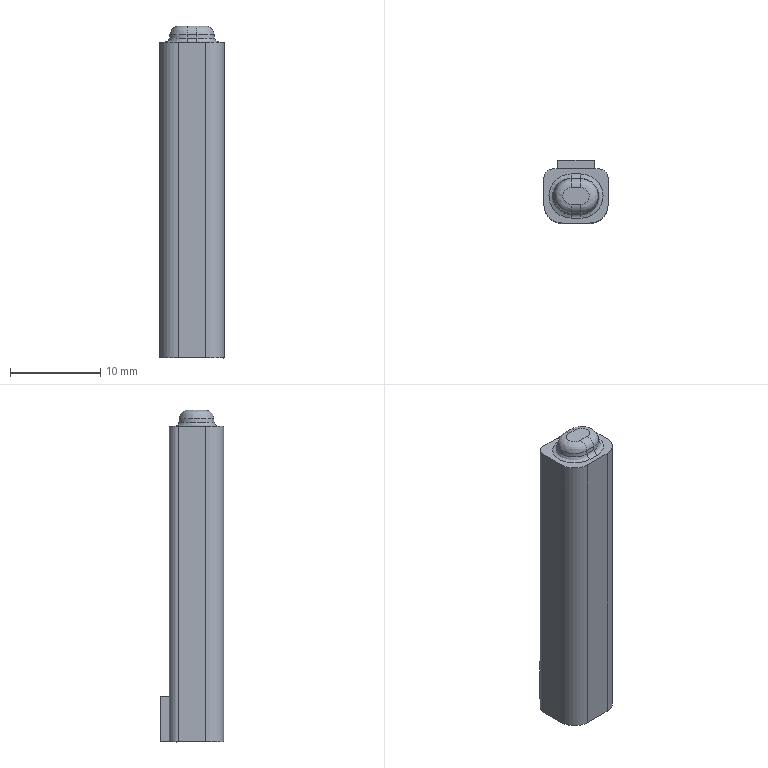Part | NX | features DIE-100 2 | 1 solid | 27 faces | box 7.1 x 7 x 36.8 mm | volume 1462 mm3 | plane 13 | cylinder 8 | spline 6 | commonest cylinder face diameters 2 x4 1 x2 4 x2
STEP:
#1=CARTESIAN_POINT('',(4190.723,-837.209,859.603));
#2=VERTEX_POINT('',#1);
#3=CARTESIAN_POINT('',(4190.723,-837.172,859.173));
#4=VERTEX_POINT('',#3);
#5=CARTESIAN_POINT('',(4190.723,-837.132,858.716));
#6=DIRECTION('',(0.,-0.08716,0.9962));
#7=VECTOR('',#6,1000.);
#8=LINE('',#5,#7);
#9=EDGE_CURVE('',#2,#4,#8,.F.);
#10=ORIENTED_EDGE('',*,*,#9,.F.);
#11=CARTESIAN_POINT('',(4190.786,-841.034,859.603));
#12=VERTEX_POINT('',#11);
#13=CARTESIAN_POINT('',(4190.723,-837.209,859.603));
#14=CARTESIAN_POINT('',(4191.232,-837.21,859.603));
#15=CARTESIAN_POINT('',(4192.249,-837.576,859.603));
#16=CARTESIAN_POINT('',(4192.911,-839.092,859.603));
#17=CARTESIAN_POINT('',(4192.297,-840.61,859.603));
#18=CARTESIAN_POINT('',(4191.295,-841.034,859.603));
#19=CARTESIAN_POINT('',(4190.786,-841.034,859.603));
#20=B_SPLINE_CURVE_WITH_KNOTS('',3,(#13,#14,#15,#16,#17,#18,#19),.UNSPECIFIED.,.F.,.F.,(4,1,1,1,4),(0.,0.001527,0.003054,0.004581,0.006107),.UNSPECIFIED.);
#21=EDGE_CURVE('',#2,#12,#20,.T.);
#22=ORIENTED_EDGE('',*,*,#21,.T.);
#23=CARTESIAN_POINT('',(4190.786,-841.072,859.173));
#24=VERTEX_POINT('',#23);
#25=CARTESIAN_POINT('',(4190.786,-841.112,858.716));
#26=DIRECTION('',(0.000000005,-0.08716,-0.9962));
#27=VECTOR('',#26,1000.);
#28=LINE('',#25,#27);
#29=EDGE_CURVE('',#12,#24,#28,.T.);
#30=ORIENTED_EDGE('',*,*,#29,.T.);
#31=CARTESIAN_POINT('',(4190.786,-841.072,859.173));
#32=CARTESIAN_POINT('',(4191.307,-841.072,859.173));
#33=CARTESIAN_POINT('',(4192.33,-840.638,859.173));
#34=CARTESIAN_POINT('',(4192.953,-839.087,859.173));
#35=CARTESIAN_POINT('',(4192.275,-837.544,859.173));
#36=CARTESIAN_POINT('',(4191.241,-837.172,859.173));
#37=CARTESIAN_POINT('',(4190.723,-837.172,859.173));
#38=B_SPLINE_CURVE_WITH_KNOTS('',3,(#31,#32,#33,#34,#35,#36,#37),.UNSPECIFIED.,.F.,.F.,(4,1,1,1,4),(-0.00000006,0.001562,0.003124,0.004686,0.006248),.UNSPECIFIED.);
#39=EDGE_CURVE('',#24,#4,#38,.T.);
#40=ORIENTED_EDGE('',*,*,#39,.T.);
#41=EDGE_LOOP('',(#10,#22,#30,#40));
#42=FACE_BOUND('',#41,.T.);
#43=CARTESIAN_POINT('',(4190.721,-837.171,859.17));
#44=CARTESIAN_POINT('',(4190.982,-837.171,859.17));
#45=CARTESIAN_POINT('',(4191.238,-837.208,859.17));
#46=CARTESIAN_POINT('',(4191.722,-837.392,859.17));
#47=CARTESIAN_POINT('',(4191.943,-837.531,859.17));
#48=CARTESIAN_POINT('',(4192.504,-838.063,859.17));
#49=CARTESIAN_POINT('',(4192.727,-838.575,859.17));
#50=CARTESIAN_POINT('',(4192.746,-839.599,859.17));
#51=CARTESIAN_POINT('',(4192.54,-840.118,859.17));
#52=CARTESIAN_POINT('',(4191.816,-840.857,859.17));
#53=CARTESIAN_POINT('',(4191.305,-841.072,859.17));
#54=CARTESIAN_POINT('',(4190.786,-841.072,859.17));
#55=CARTESIAN_POINT('',(4190.721,-837.21,859.606));
#56=CARTESIAN_POINT('',(4190.979,-837.21,859.606));
#57=CARTESIAN_POINT('',(4191.229,-837.245,859.606));
#58=CARTESIAN_POINT('',(4191.703,-837.426,859.606));
#59=CARTESIAN_POINT('',(4191.92,-837.562,859.606));
#60=CARTESIAN_POINT('',(4192.47,-838.084,859.606));
#61=CARTESIAN_POINT('',(4192.689,-838.586,859.606));
#62=CARTESIAN_POINT('',(4192.707,-839.59,859.606));
#63=CARTESIAN_POINT('',(4192.506,-840.099,859.606));
#64=CARTESIAN_POINT('',(4191.796,-840.823,859.606));
#65=CARTESIAN_POINT('',(4191.295,-841.034,859.606));
#66=CARTESIAN_POINT('',(4190.786,-841.034,859.606));
#67=B_SPLINE_SURFACE_WITH_KNOTS('',1,3,((#43,#44,#45,#46,#47,#48,#49,#50,#51,#52,#53,#54),(#55,#56,#57,#58,#59,#60,#61,#62,#63,#64,#65,#66)),.RULED_SURF.,.F.,.F.,.F.,(2,2),(4,2,2,2,2,4),(0.1782,0.3496),(0.,0.000784,0.001568,0.003136,0.004704,0.006272),.UNSPECIFIED.);
#68=ADVANCED_FACE('',(#42),#67,.T.);
#69=CARTESIAN_POINT('',(4189.687,-841.034,859.603));
#70=VERTEX_POINT('',#69);
#71=CARTESIAN_POINT('',(4189.687,-841.071,859.173));
#72=VERTEX_POINT('',#71);
#73=CARTESIAN_POINT('',(4189.687,-841.034,859.603));
#74=CARTESIAN_POINT('',(4189.687,-841.047,859.46));
#75=CARTESIAN_POINT('',(4189.687,-841.059,859.316));
#76=CARTESIAN_POINT('',(4189.687,-841.072,859.173));
#77=B_SPLINE_CURVE_WITH_KNOTS('',3,(#73,#74,#75,#76),.UNSPECIFIED.,.F.,.F.,(4,4),(-0.0008906,-0.0004582),.UNSPECIFIED.);
#78=EDGE_CURVE('',#70,#72,#77,.T.);
#79=ORIENTED_EDGE('',*,*,#78,.F.);
#80=CARTESIAN_POINT('',(4189.686,-837.209,859.603));
#81=VERTEX_POINT('',#80);
#82=CARTESIAN_POINT('',(4189.687,-841.033,859.603));
#83=CARTESIAN_POINT('',(4189.183,-841.022,859.603));
#84=CARTESIAN_POINT('',(4188.189,-840.626,859.604));
#85=CARTESIAN_POINT('',(4187.566,-839.119,859.603));
#86=CARTESIAN_POINT('',(4188.189,-837.624,859.603));
#87=CARTESIAN_POINT('',(4189.182,-837.209,859.603));
#88=CARTESIAN_POINT('',(4189.686,-837.209,859.603));
#89=B_SPLINE_CURVE_WITH_KNOTS('',3,(#82,#83,#84,#85,#86,#87,#88),.UNSPECIFIED.,.F.,.F.,(4,1,1,1,4),(0.,0.001512,0.003025,0.004537,0.00605),.UNSPECIFIED.);
#90=EDGE_CURVE('',#70,#81,#89,.T.);
#91=ORIENTED_EDGE('',*,*,#90,.T.);
#92=CARTESIAN_POINT('',(4189.686,-837.172,859.173));
#93=VERTEX_POINT('',#92);
#94=CARTESIAN_POINT('',(4189.686,-837.132,858.716));
#95=DIRECTION('',(0.000000001,0.08716,-0.9962));
#96=VECTOR('',#95,1000.);
#97=LINE('',#94,#96);
#98=EDGE_CURVE('',#81,#93,#97,.T.);
#99=ORIENTED_EDGE('',*,*,#98,.T.);
#100=CARTESIAN_POINT('',(4189.686,-837.172,859.173));
#101=CARTESIAN_POINT('',(4189.178,-837.172,859.173));
#102=CARTESIAN_POINT('',(4188.158,-837.595,859.173));
#103=CARTESIAN_POINT('',(4187.525,-839.117,859.173));
#104=CARTESIAN_POINT('',(4188.158,-840.655,859.173));
#105=CARTESIAN_POINT('',(4189.172,-841.059,859.173));
#106=CARTESIAN_POINT('',(4189.686,-841.071,859.173));
#107=B_SPLINE_CURVE_WITH_KNOTS('',3,(#100,#101,#102,#103,#104,#105,#106),.UNSPECIFIED.,.F.,.F.,(4,1,1,1,4),(-0.00000006,0.001523,0.003046,0.00457,0.006093),.UNSPECIFIED.);
#108=EDGE_CURVE('',#93,#72,#107,.T.);
#109=ORIENTED_EDGE('',*,*,#108,.T.);
#110=EDGE_LOOP('',(#79,#91,#99,#109));
#111=FACE_BOUND('',#110,.T.);
#112=CARTESIAN_POINT('',(4189.723,-841.072,859.17));
#113=CARTESIAN_POINT('',(4189.472,-841.069,859.17));
#114=CARTESIAN_POINT('',(4189.226,-841.033,859.17));
#115=CARTESIAN_POINT('',(4188.75,-840.851,859.17));
#116=CARTESIAN_POINT('',(4188.529,-840.713,859.17));
#117=CARTESIAN_POINT('',(4187.969,-840.18,859.17));
#118=CARTESIAN_POINT('',(4187.746,-839.668,859.17));
#119=CARTESIAN_POINT('',(4187.727,-838.644,859.17));
#120=CARTESIAN_POINT('',(4187.932,-838.125,859.17));
#121=CARTESIAN_POINT('',(4188.656,-837.386,859.17));
#122=CARTESIAN_POINT('',(4189.167,-837.171,859.17));
#123=CARTESIAN_POINT('',(4189.686,-837.171,859.17));
#124=CARTESIAN_POINT('',(4189.724,-841.034,859.606));
#125=CARTESIAN_POINT('',(4189.476,-841.031,859.606));
#126=CARTESIAN_POINT('',(4189.235,-840.995,859.606));
#127=CARTESIAN_POINT('',(4188.769,-840.817,859.606));
#128=CARTESIAN_POINT('',(4188.552,-840.681,859.606));
#129=CARTESIAN_POINT('',(4188.002,-840.16,859.606));
#130=CARTESIAN_POINT('',(4187.784,-839.657,859.606));
#131=CARTESIAN_POINT('',(4187.765,-838.654,859.606));
#132=CARTESIAN_POINT('',(4187.967,-838.144,859.606));
#133=CARTESIAN_POINT('',(4188.676,-837.421,859.606));
#134=CARTESIAN_POINT('',(4189.177,-837.21,859.606));
#135=CARTESIAN_POINT('',(4189.686,-837.21,859.606));
#136=B_SPLINE_SURFACE_WITH_KNOTS('',1,3,((#112,#113,#114,#115,#116,#117,#118,#119,#120,#121,#122,#123),(#124,#125,#126,#127,#128,#129,#130,#131,#132,#133,#134,#135)),.RULED_SURF.,.F.,.F.,.F.,(2,2),(4,2,2,2,2,4),(0.1782,0.3496),(0.00002755,0.000784,0.001568,0.003136,0.004704,0.006272),.UNSPECIFIED.);
#137=ADVANCED_FACE('',(#111),#136,.T.);
#138=ORIENTED_EDGE('',*,*,#98,.F.);
#139=CARTESIAN_POINT('',(4190.236,-837.209,859.603));
#140=DIRECTION('',(1.,0.,0.));
#141=VECTOR('',#140,1000.);
#142=LINE('',#139,#141);
#143=EDGE_CURVE('',#81,#2,#142,.T.);
#144=ORIENTED_EDGE('',*,*,#143,.T.);
#145=ORIENTED_EDGE('',*,*,#9,.T.);
#146=CARTESIAN_POINT('',(4190.236,-837.172,859.173));
#147=DIRECTION('',(-1.,0.,0.));
#148=VECTOR('',#147,1000.);
#149=LINE('',#146,#148);
#150=EDGE_CURVE('',#4,#93,#149,.T.);
#151=ORIENTED_EDGE('',*,*,#150,.T.);
#152=EDGE_LOOP('',(#138,#144,#145,#151));
#153=FACE_BOUND('',#152,.T.);
#154=CARTESIAN_POINT('',(4190.236,-837.132,858.716));
#155=DIRECTION('',(0.,0.9962,0.08716));
#156=DIRECTION('',(0.,-0.08716,0.9962));
#157=AXIS2_PLACEMENT_3D('',#154,#155,#156);
#158=PLANE('',#157);
#159=ADVANCED_FACE('',(#153),#158,.T.);
#160=ORIENTED_EDGE('',*,*,#29,.F.);
#161=CARTESIAN_POINT('',(4190.236,-841.034,859.603));
#162=DIRECTION('',(1.,0.,0.));
#163=VECTOR('',#162,1000.);
#164=LINE('',#161,#163);
#165=EDGE_CURVE('',#12,#70,#164,.F.);
#166=ORIENTED_EDGE('',*,*,#165,.T.);
#167=ORIENTED_EDGE('',*,*,#78,.T.);
#168=CARTESIAN_POINT('',(4190.236,-841.072,859.173));
#169=DIRECTION('',(1.,0.,0.));
#170=VECTOR('',#169,1000.);
#171=LINE('',#168,#170);
#172=EDGE_CURVE('',#72,#24,#171,.T.);
#173=ORIENTED_EDGE('',*,*,#172,.T.);
#174=EDGE_LOOP('',(#160,#166,#167,#173));
#175=FACE_BOUND('',#174,.T.);
#176=CARTESIAN_POINT('',(4190.236,-841.112,858.716));
#177=DIRECTION('',(0.,-0.9962,0.08716));
#178=DIRECTION('',(0.,-0.08716,-0.9962));
#179=AXIS2_PLACEMENT_3D('',#176,#177,#178);
#180=PLANE('',#179);
#181=ADVANCED_FACE('',(#175),#180,.T.);
#182=CARTESIAN_POINT('',(4189.686,-838.205,860.516));
#183=VERTEX_POINT('',#182);
#184=CARTESIAN_POINT('',(4189.71,-840.038,860.516));
#185=VERTEX_POINT('',#184);
#186=CARTESIAN_POINT('',(4189.686,-838.205,860.516));
#187=CARTESIAN_POINT('',(4189.198,-838.205,860.516));
#188=CARTESIAN_POINT('',(4188.556,-838.882,860.516));
#189=CARTESIAN_POINT('',(4188.983,-839.862,860.516));
#190=CARTESIAN_POINT('',(4189.468,-840.032,860.516));
#191=CARTESIAN_POINT('',(4189.71,-840.037,860.516));
#192=B_SPLINE_CURVE_WITH_KNOTS('',3,(#186,#187,#188,#189,#190,#191),.UNSPECIFIED.,.F.,.F.,(4,1,1,4),(0.,0.001465,0.002197,0.00293),.UNSPECIFIED.);
#193=EDGE_CURVE('',#183,#185,#192,.T.);
#194=ORIENTED_EDGE('',*,*,#193,.T.);
#195=CARTESIAN_POINT('',(4190.786,-840.038,860.516));
#196=VERTEX_POINT('',#195);
#197=CARTESIAN_POINT('',(4187.646,-840.038,860.516));
#198=DIRECTION('',(-1.,0.,0.));
#199=VECTOR('',#198,1000.);
#200=LINE('',#197,#199);
#201=EDGE_CURVE('',#185,#196,#200,.F.);
#202=ORIENTED_EDGE('',*,*,#201,.T.);
#203=CARTESIAN_POINT('',(4190.722,-838.205,860.516));
#204=VERTEX_POINT('',#203);
#205=CARTESIAN_POINT('',(4190.786,-840.038,860.516));
#206=CARTESIAN_POINT('',(4191.281,-840.038,860.516));
#207=CARTESIAN_POINT('',(4191.927,-839.343,860.516));
#208=CARTESIAN_POINT('',(4191.466,-838.355,860.516));
#209=CARTESIAN_POINT('',(4190.968,-838.206,860.516));
#210=CARTESIAN_POINT('',(4190.722,-838.205,860.516));
#211=B_SPLINE_CURVE_WITH_KNOTS('',3,(#205,#206,#207,#208,#209,#210),.UNSPECIFIED.,.F.,.F.,(4,1,1,4),(0.,0.001484,0.002226,0.002968),.UNSPECIFIED.);
#212=EDGE_CURVE('',#196,#204,#211,.T.);
#213=ORIENTED_EDGE('',*,*,#212,.T.);
#214=CARTESIAN_POINT('',(4187.646,-838.205,860.516));
#215=DIRECTION('',(-1.,0.,0.));
#216=VECTOR('',#215,1000.);
#217=LINE('',#214,#216);
#218=EDGE_CURVE('',#204,#183,#217,.T.);
#219=ORIENTED_EDGE('',*,*,#218,.T.);
#220=EDGE_LOOP('',(#194,#202,#213,#219));
#221=FACE_BOUND('',#220,.T.);
#222=CARTESIAN_POINT('',(4187.646,-839.12,860.516));
#223=DIRECTION('',(0.,0.,-1.));
#224=DIRECTION('',(-1.,0.,0.));
#225=AXIS2_PLACEMENT_3D('',#222,#223,#224);
#226=PLANE('',#225);
#227=ADVANCED_FACE('',(#221),#226,.F.);
#228=CARTESIAN_POINT('',(4190.723,-836.674,858.716));
#229=VERTEX_POINT('',#228);
#230=CARTESIAN_POINT('',(4190.786,-841.57,858.716));
#231=VERTEX_POINT('',#230);
#232=CARTESIAN_POINT('',(4190.723,-836.674,858.716));
#233=CARTESIAN_POINT('',(4191.373,-836.674,858.716));
#234=CARTESIAN_POINT('',(4192.664,-837.153,858.716));
#235=CARTESIAN_POINT('',(4193.505,-839.086,858.716));
#236=CARTESIAN_POINT('',(4192.72,-841.027,858.716));
#237=CARTESIAN_POINT('',(4191.439,-841.57,858.716));
#238=CARTESIAN_POINT('',(4190.786,-841.57,858.716));
#239=B_SPLINE_CURVE_WITH_KNOTS('',3,(#232,#233,#234,#235,#236,#237,#238),.UNSPECIFIED.,.F.,.F.,(4,1,1,1,4),(0.,0.001922,0.003843,0.005765,0.007686),.UNSPECIFIED.);
#240=EDGE_CURVE('',#229,#231,#239,.T.);
#241=ORIENTED_EDGE('',*,*,#240,.T.);
#242=CARTESIAN_POINT('',(4189.687,-841.57,858.716));
#243=VERTEX_POINT('',#242);
#244=CARTESIAN_POINT('',(4190.236,-841.57,858.716));
#245=DIRECTION('',(-1.,0.,0.));
#246=VECTOR('',#245,1000.);
#247=LINE('',#244,#246);
#248=EDGE_CURVE('',#231,#243,#247,.T.);
#249=ORIENTED_EDGE('',*,*,#248,.T.);
#250=CARTESIAN_POINT('',(4189.686,-836.674,858.716));
#251=VERTEX_POINT('',#250);
#252=CARTESIAN_POINT('',(4189.687,-841.569,858.716));
#253=CARTESIAN_POINT('',(4189.041,-841.557,858.716));
#254=CARTESIAN_POINT('',(4187.769,-841.046,858.716));
#255=CARTESIAN_POINT('',(4186.972,-839.117,858.716));
#256=CARTESIAN_POINT('',(4187.771,-837.205,858.716));
#257=CARTESIAN_POINT('',(4189.039,-836.674,858.716));
#258=CARTESIAN_POINT('',(4189.686,-836.674,858.716));
#259=B_SPLINE_CURVE_WITH_KNOTS('',3,(#252,#253,#254,#255,#256,#257,#258),.UNSPECIFIED.,.F.,.F.,(4,1,1,1,4),(0.,0.001938,0.003876,0.005815,0.007753),.UNSPECIFIED.);
#260=EDGE_CURVE('',#243,#251,#259,.T.);
#261=ORIENTED_EDGE('',*,*,#260,.T.);
#262=CARTESIAN_POINT('',(4190.236,-836.674,858.716));
#263=DIRECTION('',(1.,0.,0.));
#264=VECTOR('',#263,1000.);
#265=LINE('',#262,#264);
#266=EDGE_CURVE('',#251,#229,#265,.T.);
#267=ORIENTED_EDGE('',*,*,#266,.T.);
#268=EDGE_LOOP('',(#241,#249,#261,#267));
#269=FACE_BOUND('',#268,.T.);
#270=CARTESIAN_POINT('',(4190.786,-836.122,858.716));
#271=VERTEX_POINT('',#270);
#272=CARTESIAN_POINT('',(4192.786,-836.122,858.716));
#273=VERTEX_POINT('',#272);
#274=CARTESIAN_POINT('',(4190.236,-836.122,858.716));
#275=DIRECTION('',(-1.,0.,0.));
#276=VECTOR('',#275,1000.);
#277=LINE('',#274,#276);
#278=EDGE_CURVE('',#271,#273,#277,.F.);
#279=ORIENTED_EDGE('',*,*,#278,.F.);
#280=CARTESIAN_POINT('',(4189.686,-836.122,858.716));
#281=VERTEX_POINT('',#280);
#282=CARTESIAN_POINT('',(4217.236,-836.122,858.716));
#283=DIRECTION('',(1.,0.,0.));
#284=VECTOR('',#283,1000.);
#285=LINE('',#282,#284);
#286=EDGE_CURVE('',#281,#271,#285,.T.);
#287=ORIENTED_EDGE('',*,*,#286,.F.);
#288=CARTESIAN_POINT('',(4187.686,-836.122,858.716));
#289=VERTEX_POINT('',#288);
#290=CARTESIAN_POINT('',(4190.236,-836.122,858.716));
#291=DIRECTION('',(-1.,0.,0.));
#292=VECTOR('',#291,1000.);
#293=LINE('',#290,#292);
#294=EDGE_CURVE('',#289,#281,#293,.F.);
#295=ORIENTED_EDGE('',*,*,#294,.F.);
#296=CARTESIAN_POINT('',(4186.686,-837.122,858.716));
#297=VERTEX_POINT('',#296);
#298=CARTESIAN_POINT('',(4187.686,-837.122,858.716));
#299=DIRECTION('',(0.,0.,-1.));
#300=DIRECTION('',(1.,0.,0.));
#301=AXIS2_PLACEMENT_3D('',#298,#299,#300);
#302=CIRCLE('',#301,1.);
#303=EDGE_CURVE('',#297,#289,#302,.T.);
#304=ORIENTED_EDGE('',*,*,#303,.F.);
#305=CARTESIAN_POINT('',(4186.686,-840.122,858.716));
#306=VERTEX_POINT('',#305);
#307=CARTESIAN_POINT('',(4186.686,-839.122,858.716));
#308=DIRECTION('',(0.,-1.,0.));
#309=VECTOR('',#308,1000.);
#310=LINE('',#307,#309);
#311=EDGE_CURVE('',#297,#306,#310,.T.);
#312=ORIENTED_EDGE('',*,*,#311,.T.);
#313=CARTESIAN_POINT('',(4188.686,-842.122,858.716));
#314=VERTEX_POINT('',#313);
#315=CARTESIAN_POINT('',(4188.686,-840.122,858.716));
#316=DIRECTION('',(0.,0.,-1.));
#317=DIRECTION('',(1.,0.,0.));
#318=AXIS2_PLACEMENT_3D('',#315,#316,#317);
#319=CIRCLE('',#318,2.);
#320=EDGE_CURVE('',#314,#306,#319,.T.);
#321=ORIENTED_EDGE('',*,*,#320,.F.);
#322=CARTESIAN_POINT('',(4189.686,-842.122,858.716));
#323=VERTEX_POINT('',#322);
#324=CARTESIAN_POINT('',(4190.236,-842.122,858.716));
#325=DIRECTION('',(1.,0.,0.));
#326=VECTOR('',#325,1000.);
#327=LINE('',#324,#326);
#328=EDGE_CURVE('',#314,#323,#327,.T.);
#329=ORIENTED_EDGE('',*,*,#328,.T.);
#330=CARTESIAN_POINT('',(4190.786,-842.122,858.716));
#331=VERTEX_POINT('',#330);
#332=CARTESIAN_POINT('',(4189.736,-842.122,858.716));
#333=DIRECTION('',(1.,0.,0.));
#334=VECTOR('',#333,1000.);
#335=LINE('',#332,#334);
#336=EDGE_CURVE('',#323,#331,#335,.T.);
#337=ORIENTED_EDGE('',*,*,#336,.T.);
#338=CARTESIAN_POINT('',(4191.786,-842.122,858.716));
#339=VERTEX_POINT('',#338);
#340=CARTESIAN_POINT('',(4190.236,-842.122,858.716));
#341=DIRECTION('',(1.,0.,0.));
#342=VECTOR('',#341,1000.);
#343=LINE('',#340,#342);
#344=EDGE_CURVE('',#331,#339,#343,.T.);
#345=ORIENTED_EDGE('',*,*,#344,.T.);
#346=CARTESIAN_POINT('',(4193.786,-840.122,858.716));
#347=VERTEX_POINT('',#346);
#348=CARTESIAN_POINT('',(4191.786,-840.122,858.716));
#349=DIRECTION('',(0.,0.,-1.));
#350=DIRECTION('',(1.,0.,0.));
#351=AXIS2_PLACEMENT_3D('',#348,#349,#350);
#352=CIRCLE('',#351,2.);
#353=EDGE_CURVE('',#347,#339,#352,.T.);
#354=ORIENTED_EDGE('',*,*,#353,.F.);
#355=CARTESIAN_POINT('',(4193.786,-837.122,858.716));
#356=VERTEX_POINT('',#355);
#357=CARTESIAN_POINT('',(4193.786,-839.122,858.716));
#358=DIRECTION('',(0.,1.,0.));
#359=VECTOR('',#358,1000.);
#360=LINE('',#357,#359);
#361=EDGE_CURVE('',#347,#356,#360,.T.);
#362=ORIENTED_EDGE('',*,*,#361,.T.);
#363=CARTESIAN_POINT('',(4192.786,-837.122,858.716));
#364=DIRECTION('',(0.,0.,-1.));
#365=DIRECTION('',(1.,0.,0.));
#366=AXIS2_PLACEMENT_3D('',#363,#364,#365);
#367=CIRCLE('',#366,1.);
#368=EDGE_CURVE('',#273,#356,#367,.T.);
#369=ORIENTED_EDGE('',*,*,#368,.F.);
#370=EDGE_LOOP('',(#279,#287,#295,#304,#312,#321,#329,#337,#345,#354,#362,#369));
#371=FACE_BOUND('',#370,.T.);
#372=CARTESIAN_POINT('',(4190.236,-839.122,858.716));
#373=DIRECTION('',(0.,0.,1.));
#374=DIRECTION('',(1.,0.,0.));
#375=AXIS2_PLACEMENT_3D('',#372,#373,#374);
#376=PLANE('',#375);
#377=ADVANCED_FACE('',(#269,#371),#376,.T.);
#378=CARTESIAN_POINT('',(4192.236,-836.122,823.716));
#379=VERTEX_POINT('',#378);
#380=CARTESIAN_POINT('',(4192.786,-836.122,823.716));
#381=VERTEX_POINT('',#380);
#382=CARTESIAN_POINT('',(4190.736,-836.122,823.716));
#383=DIRECTION('',(1.,0.,0.));
#384=VECTOR('',#383,1000.);
#385=LINE('',#382,#384);
#386=EDGE_CURVE('',#379,#381,#385,.T.);
#387=ORIENTED_EDGE('',*,*,#386,.T.);
#388=CARTESIAN_POINT('',(4193.786,-837.122,823.716));
#389=VERTEX_POINT('',#388);
#390=CARTESIAN_POINT('',(4192.786,-837.122,823.716));
#391=DIRECTION('',(0.,0.,1.));
#392=DIRECTION('',(-1.,0.,0.));
#393=AXIS2_PLACEMENT_3D('',#390,#391,#392);
#394=CIRCLE('',#393,1.);
#395=EDGE_CURVE('',#381,#389,#394,.F.);
#396=ORIENTED_EDGE('',*,*,#395,.T.);
#397=CARTESIAN_POINT('',(4193.786,-840.122,823.716));
#398=VERTEX_POINT('',#397);
#399=CARTESIAN_POINT('',(4193.786,-839.122,823.716));
#400=DIRECTION('',(0.,-1.,0.));
#401=VECTOR('',#400,1000.);
#402=LINE('',#399,#401);
#403=EDGE_CURVE('',#389,#398,#402,.T.);
#404=ORIENTED_EDGE('',*,*,#403,.T.);
#405=CARTESIAN_POINT('',(4191.786,-842.122,823.716));
#406=VERTEX_POINT('',#405);
#407=CARTESIAN_POINT('',(4191.786,-840.122,823.716));
#408=DIRECTION('',(0.,0.,1.));
#409=DIRECTION('',(-1.,0.,0.));
#410=AXIS2_PLACEMENT_3D('',#407,#408,#409);
#411=CIRCLE('',#410,2.);
#412=EDGE_CURVE('',#406,#398,#411,.T.);
#413=ORIENTED_EDGE('',*,*,#412,.F.);
#414=CARTESIAN_POINT('',(4190.786,-842.122,823.716));
#415=VERTEX_POINT('',#414);
#416=CARTESIAN_POINT('',(4190.236,-842.122,823.716));
#417=DIRECTION('',(-1.,0.,0.));
#418=VECTOR('',#417,1000.);
#419=LINE('',#416,#418);
#420=EDGE_CURVE('',#415,#406,#419,.F.);
#421=ORIENTED_EDGE('',*,*,#420,.F.);
#422=CARTESIAN_POINT('',(4189.686,-842.122,823.716));
#423=VERTEX_POINT('',#422);
#424=CARTESIAN_POINT('',(4187.646,-842.122,823.716));
#425=DIRECTION('',(1.,0.,0.));
#426=VECTOR('',#425,1000.);
#427=LINE('',#424,#426);
#428=EDGE_CURVE('',#423,#415,#427,.T.);
#429=ORIENTED_EDGE('',*,*,#428,.F.);
#430=CARTESIAN_POINT('',(4188.686,-842.122,823.716));
#431=VERTEX_POINT('',#430);
#432=CARTESIAN_POINT('',(4190.236,-842.122,823.716));
#433=DIRECTION('',(-1.,0.,0.));
#434=VECTOR('',#433,1000.);
#435=LINE('',#432,#434);
#436=EDGE_CURVE('',#431,#423,#435,.F.);
#437=ORIENTED_EDGE('',*,*,#436,.F.);
#438=CARTESIAN_POINT('',(4186.686,-840.122,823.716));
#439=VERTEX_POINT('',#438);
#440=CARTESIAN_POINT('',(4188.686,-840.122,823.716));
#441=DIRECTION('',(0.,0.,1.));
#442=DIRECTION('',(-1.,0.,0.));
#443=AXIS2_PLACEMENT_3D('',#440,#441,#442);
#444=CIRCLE('',#443,2.);
#445=EDGE_CURVE('',#439,#431,#444,.T.);
#446=ORIENTED_EDGE('',*,*,#445,.F.);
#447=CARTESIAN_POINT('',(4186.686,-837.122,823.716));
#448=VERTEX_POINT('',#447);
#449=CARTESIAN_POINT('',(4186.686,-839.122,823.716));
#450=DIRECTION('',(0.,1.,0.));
#451=VECTOR('',#450,1000.);
#452=LINE('',#449,#451);
#453=EDGE_CURVE('',#439,#448,#452,.T.);
#454=ORIENTED_EDGE('',*,*,#453,.T.);
#455=CARTESIAN_POINT('',(4187.686,-836.122,823.716));
#456=VERTEX_POINT('',#455);
#457=CARTESIAN_POINT('',(4187.686,-837.122,823.716));
#458=DIRECTION('',(0.,0.,1.));
#459=DIRECTION('',(-1.,0.,0.));
#460=AXIS2_PLACEMENT_3D('',#457,#458,#459);
#461=CIRCLE('',#460,1.);
#462=EDGE_CURVE('',#456,#448,#461,.T.);
#463=ORIENTED_EDGE('',*,*,#462,.F.);
#464=CARTESIAN_POINT('',(4188.236,-836.122,823.716));
#465=VERTEX_POINT('',#464);
#466=CARTESIAN_POINT('',(4190.736,-836.122,823.716));
#467=DIRECTION('',(1.,0.,0.));
#468=VECTOR('',#467,1000.);
#469=LINE('',#466,#468);
#470=EDGE_CURVE('',#456,#465,#469,.T.);
#471=ORIENTED_EDGE('',*,*,#470,.T.);
#472=CARTESIAN_POINT('',(4188.236,-835.122,823.716));
#473=VERTEX_POINT('',#472);
#474=CARTESIAN_POINT('',(4188.236,-1716.244,823.716));
#475=DIRECTION('',(0.,-1.,0.));
#476=VECTOR('',#475,1000.);
#477=LINE('',#474,#476);
#478=EDGE_CURVE('',#473,#465,#477,.T.);
#479=ORIENTED_EDGE('',*,*,#478,.F.);
#480=CARTESIAN_POINT('',(4192.236,-835.122,823.716));
#481=VERTEX_POINT('',#480);
#482=CARTESIAN_POINT('',(4192.786,-835.122,823.716));
#483=DIRECTION('',(-1.,0.,0.));
#484=VECTOR('',#483,1000.);
#485=LINE('',#482,#484);
#486=EDGE_CURVE('',#481,#473,#485,.T.);
#487=ORIENTED_EDGE('',*,*,#486,.F.);
#488=CARTESIAN_POINT('',(4192.236,-1716.244,823.716));
#489=DIRECTION('',(0.,1.,0.));
#490=VECTOR('',#489,1000.);
#491=LINE('',#488,#490);
#492=EDGE_CURVE('',#379,#481,#491,.T.);
#493=ORIENTED_EDGE('',*,*,#492,.F.);
#494=EDGE_LOOP('',(#387,#396,#404,#413,#421,#429,#437,#446,#454,#463,#471,#479,#487,#493));
#495=FACE_BOUND('',#494,.T.);
#496=CARTESIAN_POINT('',(4187.646,-839.12,823.716));
#497=DIRECTION('',(0.,0.,-1.));
#498=DIRECTION('',(-1.,0.,0.));
#499=AXIS2_PLACEMENT_3D('',#496,#497,#498);
#500=PLANE('',#499);
#501=ADVANCED_FACE('',(#495),#500,.T.);
#502=ORIENTED_EDGE('',*,*,#344,.F.);
#503=ORIENTED_EDGE('',*,*,#336,.F.);
#504=ORIENTED_EDGE('',*,*,#328,.F.);
#505=CARTESIAN_POINT('',(4188.686,-842.122,823.716));
#506=DIRECTION('',(0.,0.,1.));
#507=VECTOR('',#506,1000.);
#508=LINE('',#505,#507);
#509=EDGE_CURVE('',#431,#314,#508,.T.);
#510=ORIENTED_EDGE('',*,*,#509,.F.);
#511=ORIENTED_EDGE('',*,*,#436,.T.);
#512=ORIENTED_EDGE('',*,*,#428,.T.);
#513=ORIENTED_EDGE('',*,*,#420,.T.);
#514=CARTESIAN_POINT('',(4191.786,-842.122,823.716));
#515=DIRECTION('',(0.,0.,1.));
#516=VECTOR('',#515,1000.);
#517=LINE('',#514,#516);
#518=EDGE_CURVE('',#339,#406,#517,.F.);
#519=ORIENTED_EDGE('',*,*,#518,.F.);
#520=EDGE_LOOP('',(#502,#503,#504,#510,#511,#512,#513,#519));
#521=FACE_BOUND('',#520,.T.);
#522=CARTESIAN_POINT('',(4189.736,-842.122,823.716));
#523=DIRECTION('',(0.,-1.,0.));
#524=DIRECTION('',(-1.,0.,0.));
#525=AXIS2_PLACEMENT_3D('',#522,#523,#524);
#526=PLANE('',#525);
#527=ADVANCED_FACE('',(#521),#526,.T.);
#528=CARTESIAN_POINT('',(4188.236,-836.122,828.716));
#529=VERTEX_POINT('',#528);
#530=CARTESIAN_POINT('',(4188.236,-836.122,823.716));
#531=DIRECTION('',(0.,0.,-1.));
#532=VECTOR('',#531,1000.);
#533=LINE('',#530,#532);
#534=EDGE_CURVE('',#529,#465,#533,.T.);
#535=ORIENTED_EDGE('',*,*,#534,.T.);
#536=ORIENTED_EDGE('',*,*,#470,.F.);
#537=CARTESIAN_POINT('',(4187.686,-836.122,823.716));
#538=DIRECTION('',(0.,0.,1.));
#539=VECTOR('',#538,1000.);
#540=LINE('',#537,#539);
#541=EDGE_CURVE('',#289,#456,#540,.F.);
#542=ORIENTED_EDGE('',*,*,#541,.F.);
#543=ORIENTED_EDGE('',*,*,#294,.T.);
#544=ORIENTED_EDGE('',*,*,#286,.T.);
#545=ORIENTED_EDGE('',*,*,#278,.T.);
#546=CARTESIAN_POINT('',(4192.786,-836.122,823.716));
#547=DIRECTION('',(0.,0.,1.));
#548=VECTOR('',#547,1000.);
#549=LINE('',#546,#548);
#550=EDGE_CURVE('',#381,#273,#549,.T.);
#551=ORIENTED_EDGE('',*,*,#550,.F.);
#552=ORIENTED_EDGE('',*,*,#386,.F.);
#553=CARTESIAN_POINT('',(4192.236,-836.122,828.716));
#554=VERTEX_POINT('',#553);
#555=CARTESIAN_POINT('',(4192.236,-836.122,823.716));
#556=DIRECTION('',(0.,0.,1.));
#557=VECTOR('',#556,1000.);
#558=LINE('',#555,#557);
#559=EDGE_CURVE('',#379,#554,#558,.T.);
#560=ORIENTED_EDGE('',*,*,#559,.T.);
#561=CARTESIAN_POINT('',(4190.736,-836.122,828.716));
#562=DIRECTION('',(1.,0.,0.));
#563=VECTOR('',#562,1000.);
#564=LINE('',#561,#563);
#565=EDGE_CURVE('',#529,#554,#564,.T.);
#566=ORIENTED_EDGE('',*,*,#565,.F.);
#567=EDGE_LOOP('',(#535,#536,#542,#543,#544,#545,#551,#552,#560,#566));
#568=FACE_BOUND('',#567,.T.);
#569=CARTESIAN_POINT('',(4190.736,-836.122,823.716));
#570=DIRECTION('',(0.,1.,0.));
#571=DIRECTION('',(1.,0.,0.));
#572=AXIS2_PLACEMENT_3D('',#569,#570,#571);
#573=PLANE('',#572);
#574=ADVANCED_FACE('',(#568),#573,.T.);
#575=ORIENTED_EDGE('',*,*,#361,.F.);
#576=CARTESIAN_POINT('',(4193.786,-840.122,823.716));
#577=DIRECTION('',(0.,0.,1.));
#578=VECTOR('',#577,1000.);
#579=LINE('',#576,#578);
#580=EDGE_CURVE('',#398,#347,#579,.T.);
#581=ORIENTED_EDGE('',*,*,#580,.F.);
#582=ORIENTED_EDGE('',*,*,#403,.F.);
#583=CARTESIAN_POINT('',(4193.786,-837.122,823.716));
#584=DIRECTION('',(0.,0.,1.));
#585=VECTOR('',#584,1000.);
#586=LINE('',#583,#585);
#587=EDGE_CURVE('',#356,#389,#586,.F.);
#588=ORIENTED_EDGE('',*,*,#587,.F.);
#589=EDGE_LOOP('',(#575,#581,#582,#588));
#590=FACE_BOUND('',#589,.T.);
#591=CARTESIAN_POINT('',(4193.786,-839.122,823.716));
#592=DIRECTION('',(1.,0.,0.));
#593=DIRECTION('',(0.,0.,-1.));
#594=AXIS2_PLACEMENT_3D('',#591,#592,#593);
#595=PLANE('',#594);
#596=ADVANCED_FACE('',(#590),#595,.T.);
#597=ORIENTED_EDGE('',*,*,#453,.F.);
#598=CARTESIAN_POINT('',(4186.686,-840.122,823.716));
#599=DIRECTION('',(0.,0.,1.));
#600=VECTOR('',#599,1000.);
#601=LINE('',#598,#600);
#602=EDGE_CURVE('',#306,#439,#601,.F.);
#603=ORIENTED_EDGE('',*,*,#602,.F.);
#604=ORIENTED_EDGE('',*,*,#311,.F.);
#605=CARTESIAN_POINT('',(4186.686,-837.122,823.716));
#606=DIRECTION('',(0.,0.,1.));
#607=VECTOR('',#606,1000.);
#608=LINE('',#605,#607);
#609=EDGE_CURVE('',#448,#297,#608,.T.);
#610=ORIENTED_EDGE('',*,*,#609,.F.);
#611=EDGE_LOOP('',(#597,#603,#604,#610));
#612=FACE_BOUND('',#611,.T.);
#613=CARTESIAN_POINT('',(4186.686,-839.122,823.716));
#614=DIRECTION('',(-1.,0.,0.));
#615=DIRECTION('',(0.,0.,1.));
#616=AXIS2_PLACEMENT_3D('',#613,#614,#615);
#617=PLANE('',#616);
#618=ADVANCED_FACE('',(#612),#617,.T.);
#619=ORIENTED_EDGE('',*,*,#412,.T.);
#620=ORIENTED_EDGE('',*,*,#580,.T.);
#621=ORIENTED_EDGE('',*,*,#353,.T.);
#622=ORIENTED_EDGE('',*,*,#518,.T.);
#623=EDGE_LOOP('',(#619,#620,#621,#622));
#624=FACE_BOUND('',#623,.T.);
#625=CARTESIAN_POINT('',(4191.786,-840.122,823.716));
#626=DIRECTION('',(0.,0.,1.));
#627=DIRECTION('',(1.,0.,0.));
#628=AXIS2_PLACEMENT_3D('',#625,#626,#627);
#629=CYLINDRICAL_SURFACE('',#628,2.);
#630=ADVANCED_FACE('',(#624),#629,.T.);
#631=ORIENTED_EDGE('',*,*,#445,.T.);
#632=ORIENTED_EDGE('',*,*,#509,.T.);
#633=ORIENTED_EDGE('',*,*,#320,.T.);
#634=ORIENTED_EDGE('',*,*,#602,.T.);
#635=EDGE_LOOP('',(#631,#632,#633,#634));
#636=FACE_BOUND('',#635,.T.);
#637=CARTESIAN_POINT('',(4188.686,-840.122,823.716));
#638=DIRECTION('',(0.,0.,1.));
#639=DIRECTION('',(1.,0.,0.));
#640=AXIS2_PLACEMENT_3D('',#637,#638,#639);
#641=CYLINDRICAL_SURFACE('',#640,2.);
#642=ADVANCED_FACE('',(#636),#641,.T.);
#643=ORIENTED_EDGE('',*,*,#550,.T.);
#644=ORIENTED_EDGE('',*,*,#368,.T.);
#645=ORIENTED_EDGE('',*,*,#587,.T.);
#646=ORIENTED_EDGE('',*,*,#395,.F.);
#647=EDGE_LOOP('',(#643,#644,#645,#646));
#648=FACE_BOUND('',#647,.T.);
#649=CARTESIAN_POINT('',(4192.786,-837.122,823.716));
#650=DIRECTION('',(0.,0.,1.));
#651=DIRECTION('',(1.,0.,0.));
#652=AXIS2_PLACEMENT_3D('',#649,#650,#651);
#653=CYLINDRICAL_SURFACE('',#652,1.);
#654=ADVANCED_FACE('',(#648),#653,.T.);
#655=ORIENTED_EDGE('',*,*,#609,.T.);
#656=ORIENTED_EDGE('',*,*,#303,.T.);
#657=ORIENTED_EDGE('',*,*,#541,.T.);
#658=ORIENTED_EDGE('',*,*,#462,.T.);
#659=EDGE_LOOP('',(#655,#656,#657,#658));
#660=FACE_BOUND('',#659,.T.);
#661=CARTESIAN_POINT('',(4187.686,-837.122,823.716));
#662=DIRECTION('',(0.,0.,1.));
#663=DIRECTION('',(1.,0.,0.));
#664=AXIS2_PLACEMENT_3D('',#661,#662,#663);
#665=CYLINDRICAL_SURFACE('',#664,1.);
#666=ADVANCED_FACE('',(#660),#665,.T.);
#667=CARTESIAN_POINT('',(4188.236,-835.122,828.716));
#668=VERTEX_POINT('',#667);
#669=CARTESIAN_POINT('',(4188.236,-1716.244,828.716));
#670=DIRECTION('',(0.,-1.,0.));
#671=VECTOR('',#670,1000.);
#672=LINE('',#669,#671);
#673=EDGE_CURVE('',#668,#529,#672,.T.);
#674=ORIENTED_EDGE('',*,*,#673,.F.);
#675=CARTESIAN_POINT('',(4188.236,-835.122,828.716));
#676=DIRECTION('',(0.,0.,-1.));
#677=VECTOR('',#676,1000.);
#678=LINE('',#675,#677);
#679=EDGE_CURVE('',#668,#473,#678,.T.);
#680=ORIENTED_EDGE('',*,*,#679,.T.);
#681=ORIENTED_EDGE('',*,*,#478,.T.);
#682=ORIENTED_EDGE('',*,*,#534,.F.);
#683=EDGE_LOOP('',(#674,#680,#681,#682));
#684=FACE_BOUND('',#683,.T.);
#685=CARTESIAN_POINT('',(4188.236,-835.122,828.716));
#686=DIRECTION('',(-1.,0.,0.));
#687=DIRECTION('',(0.,1.,0.));
#688=AXIS2_PLACEMENT_3D('',#685,#686,#687);
#689=PLANE('',#688);
#690=ADVANCED_FACE('',(#684),#689,.T.);
#691=ORIENTED_EDGE('',*,*,#492,.T.);
#692=CARTESIAN_POINT('',(4192.236,-835.122,828.716));
#693=VERTEX_POINT('',#692);
#694=CARTESIAN_POINT('',(4192.236,-835.122,828.716));
#695=DIRECTION('',(0.,0.,-1.));
#696=VECTOR('',#695,1000.);
#697=LINE('',#694,#696);
#698=EDGE_CURVE('',#693,#481,#697,.T.);
#699=ORIENTED_EDGE('',*,*,#698,.F.);
#700=CARTESIAN_POINT('',(4192.236,-1716.244,828.716));
#701=DIRECTION('',(0.,1.,0.));
#702=VECTOR('',#701,1000.);
#703=LINE('',#700,#702);
#704=EDGE_CURVE('',#554,#693,#703,.T.);
#705=ORIENTED_EDGE('',*,*,#704,.F.);
#706=ORIENTED_EDGE('',*,*,#559,.F.);
#707=EDGE_LOOP('',(#691,#699,#705,#706));
#708=FACE_BOUND('',#707,.T.);
#709=CARTESIAN_POINT('',(4192.236,-836.172,828.716));
#710=DIRECTION('',(1.,0.,0.));
#711=DIRECTION('',(0.,-1.,0.));
#712=AXIS2_PLACEMENT_3D('',#709,#710,#711);
#713=PLANE('',#712);
#714=ADVANCED_FACE('',(#708),#713,.T.);
#715=ORIENTED_EDGE('',*,*,#486,.T.);
#716=ORIENTED_EDGE('',*,*,#679,.F.);
#717=CARTESIAN_POINT('',(4192.786,-835.122,828.716));
#718=DIRECTION('',(-1.,0.,0.));
#719=VECTOR('',#718,1000.);
#720=LINE('',#717,#719);
#721=EDGE_CURVE('',#693,#668,#720,.T.);
#722=ORIENTED_EDGE('',*,*,#721,.F.);
#723=ORIENTED_EDGE('',*,*,#698,.T.);
#724=EDGE_LOOP('',(#715,#716,#722,#723));
#725=FACE_BOUND('',#724,.T.);
#726=CARTESIAN_POINT('',(4192.786,-835.122,828.716));
#727=DIRECTION('',(0.,1.,0.));
#728=DIRECTION('',(1.,0.,0.));
#729=AXIS2_PLACEMENT_3D('',#726,#727,#728);
#730=PLANE('',#729);
#731=ADVANCED_FACE('',(#725),#730,.T.);
#732=ORIENTED_EDGE('',*,*,#565,.T.);
#733=ORIENTED_EDGE('',*,*,#704,.T.);
#734=ORIENTED_EDGE('',*,*,#721,.T.);
#735=ORIENTED_EDGE('',*,*,#673,.T.);
#736=EDGE_LOOP('',(#732,#733,#734,#735));
#737=FACE_BOUND('',#736,.T.);
#738=CARTESIAN_POINT('',(0.000000011,-1716.244,828.716));
#739=DIRECTION('',(0.,0.,-1.));
#740=DIRECTION('',(-1.,0.,0.));
#741=AXIS2_PLACEMENT_3D('',#738,#739,#740);
#742=PLANE('',#741);
#743=ADVANCED_FACE('',(#737),#742,.F.);
#744=CARTESIAN_POINT('',(4190.723,-836.674,859.216));
#745=DIRECTION('',(-1.,0.0005734,0.));
#746=DIRECTION('',(-0.0005734,-1.,0.));
#747=AXIS2_PLACEMENT_3D('',#744,#745,#746);
#748=CIRCLE('',#747,0.5);
#749=EDGE_CURVE('',#229,#4,#748,.T.);
#750=ORIENTED_EDGE('',*,*,#749,.F.);
#751=ORIENTED_EDGE('',*,*,#266,.F.);
#752=CARTESIAN_POINT('',(4189.686,-836.674,859.216));
#753=DIRECTION('',(1.,0.,0.));
#754=DIRECTION('',(0.,1.,0.));
#755=AXIS2_PLACEMENT_3D('',#752,#753,#754);
#756=CIRCLE('',#755,0.5);
#757=EDGE_CURVE('',#93,#251,#756,.T.);
#758=ORIENTED_EDGE('',*,*,#757,.F.);
#759=ORIENTED_EDGE('',*,*,#150,.F.);
#760=EDGE_LOOP('',(#750,#751,#758,#759));
#761=FACE_BOUND('',#760,.T.);
#762=CARTESIAN_POINT('',(4190.236,-836.674,859.216));
#763=DIRECTION('',(1.,0.,0.));
#764=DIRECTION('',(0.,1.,0.));
#765=AXIS2_PLACEMENT_3D('',#762,#763,#764);
#766=CYLINDRICAL_SURFACE('',#765,0.5);
#767=ADVANCED_FACE('',(#761),#766,.F.);
#768=ORIENTED_EDGE('',*,*,#757,.T.);
#769=ORIENTED_EDGE('',*,*,#260,.F.);
#770=CARTESIAN_POINT('',(4189.687,-841.072,859.173));
#771=CARTESIAN_POINT('',(4189.687,-841.093,858.926));
#772=CARTESIAN_POINT('',(4189.687,-841.323,858.716));
#773=CARTESIAN_POINT('',(4189.687,-841.57,858.716));
#774=B_SPLINE_CURVE_WITH_KNOTS('',3,(#770,#771,#772,#773),.UNSPECIFIED.,.F.,.F.,(4,4),(0.,1.),.UNSPECIFIED.);
#775=EDGE_CURVE('',#72,#243,#774,.T.);
#776=ORIENTED_EDGE('',*,*,#775,.F.);
#777=ORIENTED_EDGE('',*,*,#108,.F.);
#778=EDGE_LOOP('',(#768,#769,#776,#777));
#779=FACE_BOUND('',#778,.T.);
#780=CARTESIAN_POINT('',(4189.686,-837.172,859.173));
#781=CARTESIAN_POINT('',(4189.686,-837.132,858.716));
#782=CARTESIAN_POINT('',(4189.686,-836.674,858.716));
#783=CARTESIAN_POINT('',(4189.172,-837.172,859.173));
#784=CARTESIAN_POINT('',(4189.161,-837.132,858.716));
#785=CARTESIAN_POINT('',(4189.035,-836.674,858.716));
#786=CARTESIAN_POINT('',(4188.151,-837.6,859.173));
#787=CARTESIAN_POINT('',(4188.12,-837.569,858.716));
#788=CARTESIAN_POINT('',(4187.76,-837.211,858.716));
#789=CARTESIAN_POINT('',(4187.519,-839.138,859.173));
#790=CARTESIAN_POINT('',(4187.475,-839.138,858.716));
#791=CARTESIAN_POINT('',(4186.969,-839.142,858.716));
#792=CARTESIAN_POINT('',(4188.189,-840.679,859.173));
#793=CARTESIAN_POINT('',(4188.157,-840.711,858.716));
#794=CARTESIAN_POINT('',(4187.794,-841.076,858.716));
#795=CARTESIAN_POINT('',(4189.185,-841.069,859.173));
#796=CARTESIAN_POINT('',(4189.177,-841.109,858.716));
#797=CARTESIAN_POINT('',(4189.084,-841.566,858.716));
#798=CARTESIAN_POINT('',(4189.736,-841.072,859.173));
#799=CARTESIAN_POINT('',(4189.736,-841.112,858.716));
#800=CARTESIAN_POINT('',(4189.734,-841.57,858.716));
#801=(BOUNDED_SURFACE()B_SPLINE_SURFACE(3,2,((#780,#781,#782),(#783,#784,#785),(#786,#787,#788),(#789,#790,#791),(#792,#793,#794),(#795,#796,#797),(#798,#799,#800)),.UNSPECIFIED.,.F.,.F.,.F.)B_SPLINE_SURFACE_WITH_KNOTS((4,1,1,1,4),(3,3),(0.,0.001924,0.003849,0.005773,0.007697),(0.,1.),.UNSPECIFIED.)GEOMETRIC_REPRESENTATION_ITEM()RATIONAL_B_SPLINE_SURFACE(((1.,0.7373,1.),(1.,0.7373,1.),(1.,0.7373,1.),(1.,0.7373,1.),(1.,0.7373,1.),(1.,0.7373,1.),(1.,0.7373,1.)))REPRESENTATION_ITEM('')SURFACE());
#802=ADVANCED_FACE('',(#779),#801,.F.);
#803=ORIENTED_EDGE('',*,*,#749,.T.);
#804=ORIENTED_EDGE('',*,*,#39,.F.);
#805=CARTESIAN_POINT('',(4190.786,-841.57,859.216));
#806=DIRECTION('',(1.,-0.000000003,0.));
#807=DIRECTION('',(0.000000003,1.,0.));
#808=AXIS2_PLACEMENT_3D('',#805,#806,#807);
#809=CIRCLE('',#808,0.5);
#810=EDGE_CURVE('',#231,#24,#809,.T.);
#811=ORIENTED_EDGE('',*,*,#810,.F.);
#812=ORIENTED_EDGE('',*,*,#240,.F.);
#813=EDGE_LOOP('',(#803,#804,#811,#812));
#814=FACE_BOUND('',#813,.T.);
#815=CARTESIAN_POINT('',(4190.723,-836.674,858.716));
#816=CARTESIAN_POINT('',(4190.723,-837.132,858.716));
#817=CARTESIAN_POINT('',(4190.723,-837.172,859.173));
#818=CARTESIAN_POINT('',(4191.373,-836.674,858.716));
#819=CARTESIAN_POINT('',(4191.283,-837.132,858.716));
#820=CARTESIAN_POINT('',(4191.275,-837.172,859.173));
#821=CARTESIAN_POINT('',(4192.664,-837.153,858.716));
#822=CARTESIAN_POINT('',(4192.304,-837.522,858.716));
#823=CARTESIAN_POINT('',(4192.273,-837.554,859.173));
#824=CARTESIAN_POINT('',(4193.505,-839.086,858.716));
#825=CARTESIAN_POINT('',(4192.998,-839.093,858.716));
#826=CARTESIAN_POINT('',(4192.954,-839.094,859.173));
#827=CARTESIAN_POINT('',(4192.72,-841.027,858.716));
#828=CARTESIAN_POINT('',(4192.359,-840.671,858.716));
#829=CARTESIAN_POINT('',(4192.327,-840.64,859.173));
#830=CARTESIAN_POINT('',(4191.439,-841.57,858.716));
#831=CARTESIAN_POINT('',(4191.313,-841.112,858.716));
#832=CARTESIAN_POINT('',(4191.302,-841.072,859.173));
#833=CARTESIAN_POINT('',(4190.786,-841.57,858.716));
#834=CARTESIAN_POINT('',(4190.786,-841.112,858.716));
#835=CARTESIAN_POINT('',(4190.786,-841.072,859.173));
#836=(BOUNDED_SURFACE()B_SPLINE_SURFACE(3,2,((#815,#816,#817),(#818,#819,#820),(#821,#822,#823),(#824,#825,#826),(#827,#828,#829),(#830,#831,#832),(#833,#834,#835)),.UNSPECIFIED.,.F.,.F.,.F.)B_SPLINE_SURFACE_WITH_KNOTS((4,1,1,1,4),(3,3),(0.,0.001922,0.003843,0.005765,0.007686),(0.,1.),.UNSPECIFIED.)GEOMETRIC_REPRESENTATION_ITEM()RATIONAL_B_SPLINE_SURFACE(((1.,0.7373,1.),(1.,0.7373,1.),(1.,0.7373,1.),(1.,0.7373,1.),(1.,0.7373,1.),(1.,0.7373,1.),(1.,0.7373,1.)))REPRESENTATION_ITEM('')SURFACE());
#837=ADVANCED_FACE('',(#814),#836,.F.);
#838=ORIENTED_EDGE('',*,*,#775,.T.);
#839=ORIENTED_EDGE('',*,*,#248,.F.);
#840=ORIENTED_EDGE('',*,*,#810,.T.);
#841=ORIENTED_EDGE('',*,*,#172,.F.);
#842=EDGE_LOOP('',(#838,#839,#840,#841));
#843=FACE_BOUND('',#842,.T.);
#844=CARTESIAN_POINT('',(4190.236,-841.57,859.216));
#845=DIRECTION('',(-1.,0.,0.));
#846=DIRECTION('',(0.,-1.,0.));
#847=AXIS2_PLACEMENT_3D('',#844,#845,#846);
#848=CYLINDRICAL_SURFACE('',#847,0.5);
#849=ADVANCED_FACE('',(#843),#848,.F.);
#850=CARTESIAN_POINT('',(4190.722,-838.205,859.516));
#851=DIRECTION('',(1.,-0.0005749,0.));
#852=DIRECTION('',(0.0005749,1.,0.));
#853=AXIS2_PLACEMENT_3D('',#850,#851,#852);
#854=CIRCLE('',#853,1.);
#855=EDGE_CURVE('',#2,#204,#854,.T.);
#856=ORIENTED_EDGE('',*,*,#855,.F.);
#857=ORIENTED_EDGE('',*,*,#143,.F.);
#858=CARTESIAN_POINT('',(4189.686,-838.205,859.516));
#859=DIRECTION('',(1.,0.,0.));
#860=DIRECTION('',(0.,1.,0.));
#861=AXIS2_PLACEMENT_3D('',#858,#859,#860);
#862=CIRCLE('',#861,1.);
#863=EDGE_CURVE('',#183,#81,#862,.F.);
#864=ORIENTED_EDGE('',*,*,#863,.F.);
#865=ORIENTED_EDGE('',*,*,#218,.F.);
#866=EDGE_LOOP('',(#856,#857,#864,#865));
#867=FACE_BOUND('',#866,.T.);
#868=CARTESIAN_POINT('',(4190.236,-838.205,859.516));
#869=DIRECTION('',(-1.,0.,0.));
#870=DIRECTION('',(0.,-1.,0.));
#871=AXIS2_PLACEMENT_3D('',#868,#869,#870);
#872=CYLINDRICAL_SURFACE('',#871,1.);
#873=ADVANCED_FACE('',(#867),#872,.T.);
#874=ORIENTED_EDGE('',*,*,#863,.T.);
#875=ORIENTED_EDGE('',*,*,#90,.F.);
#876=CARTESIAN_POINT('',(4189.687,-841.034,859.603));
#877=CARTESIAN_POINT('',(4189.687,-841.019,859.781));
#878=CARTESIAN_POINT('',(4189.692,-840.886,860.211));
#879=CARTESIAN_POINT('',(4189.703,-840.354,860.516));
#880=CARTESIAN_POINT('',(4189.71,-840.037,860.516));
#881=B_SPLINE_CURVE_WITH_KNOTS('',3,(#876,#877,#878,#879,#880),.UNSPECIFIED.,.F.,.F.,(4,1,4),(0.,0.5,1.),.UNSPECIFIED.);
#882=EDGE_CURVE('',#185,#70,#881,.F.);
#883=ORIENTED_EDGE('',*,*,#882,.F.);
#884=ORIENTED_EDGE('',*,*,#193,.F.);
#885=EDGE_LOOP('',(#874,#875,#883,#884));
#886=FACE_BOUND('',#885,.T.);
#887=CARTESIAN_POINT('',(4189.71,-840.037,860.516));
#888=CARTESIAN_POINT('',(4189.689,-840.953,860.516));
#889=CARTESIAN_POINT('',(4189.687,-841.033,859.603));
#890=CARTESIAN_POINT('',(4189.589,-840.035,860.516));
#891=CARTESIAN_POINT('',(4189.5,-840.949,860.516));
#892=CARTESIAN_POINT('',(4189.493,-841.029,859.603));
#893=CARTESIAN_POINT('',(4189.347,-840.,860.516));
#894=CARTESIAN_POINT('',(4189.003,-840.879,860.516));
#895=CARTESIAN_POINT('',(4188.974,-840.956,859.603));
#896=CARTESIAN_POINT('',(4188.929,-839.733,860.516));
#897=CARTESIAN_POINT('',(4188.175,-840.344,860.516));
#898=CARTESIAN_POINT('',(4188.11,-840.398,859.603));
#899=CARTESIAN_POINT('',(4188.669,-839.135,860.516));
#900=CARTESIAN_POINT('',(4187.648,-839.15,860.516));
#901=CARTESIAN_POINT('',(4187.559,-839.151,859.603));
#902=CARTESIAN_POINT('',(4188.963,-838.408,860.516));
#903=CARTESIAN_POINT('',(4188.248,-837.695,860.516));
#904=CARTESIAN_POINT('',(4188.186,-837.633,859.603));
#905=CARTESIAN_POINT('',(4189.442,-838.205,860.516));
#906=CARTESIAN_POINT('',(4189.176,-837.289,860.516));
#907=CARTESIAN_POINT('',(4189.153,-837.209,859.603));
#908=CARTESIAN_POINT('',(4189.686,-838.205,860.516));
#909=CARTESIAN_POINT('',(4189.686,-837.289,860.516));
#910=CARTESIAN_POINT('',(4189.686,-837.209,859.603));
#911=(BOUNDED_SURFACE()B_SPLINE_SURFACE(3,2,((#887,#888,#889),(#890,#891,#892),(#893,#894,#895),(#896,#897,#898),(#899,#900,#901),(#902,#903,#904),(#905,#906,#907),(#908,#909,#910)),.UNSPECIFIED.,.F.,.F.,.F.)B_SPLINE_SURFACE_WITH_KNOTS((4,1,1,1,1,4),(3,3),(0.006239,0.006603,0.006967,0.007694,0.008421,0.009148),(0.,1.),.UNSPECIFIED.)GEOMETRIC_REPRESENTATION_ITEM()RATIONAL_B_SPLINE_SURFACE(((1.,0.7373,1.),(1.,0.7372,1.),(1.,0.7373,1.),(1.,0.7373,1.),(1.,0.7373,1.),(1.,0.7373,1.),(1.,0.7373,1.),(1.,0.7373,1.)))REPRESENTATION_ITEM('')SURFACE());
#912=ADVANCED_FACE('',(#886),#911,.T.);
#913=ORIENTED_EDGE('',*,*,#855,.T.);
#914=ORIENTED_EDGE('',*,*,#212,.F.);
#915=CARTESIAN_POINT('',(4190.786,-840.038,859.516));
#916=DIRECTION('',(-1.,0.,0.));
#917=DIRECTION('',(0.,-1.,0.));
#918=AXIS2_PLACEMENT_3D('',#915,#916,#917);
#919=CIRCLE('',#918,1.);
#920=EDGE_CURVE('',#12,#196,#919,.T.);
#921=ORIENTED_EDGE('',*,*,#920,.F.);
#922=ORIENTED_EDGE('',*,*,#21,.F.);
#923=EDGE_LOOP('',(#913,#914,#921,#922));
#924=FACE_BOUND('',#923,.T.);
#925=CARTESIAN_POINT('',(4190.722,-838.205,860.516));
#926=CARTESIAN_POINT('',(4190.723,-837.289,860.516));
#927=CARTESIAN_POINT('',(4190.723,-837.209,859.603));
#928=CARTESIAN_POINT('',(4190.968,-838.206,860.516));
#929=CARTESIAN_POINT('',(4191.094,-837.289,860.516));
#930=CARTESIAN_POINT('',(4191.105,-837.21,859.603));
#931=CARTESIAN_POINT('',(4191.468,-838.357,860.516));
#932=CARTESIAN_POINT('',(4192.173,-837.591,860.516));
#933=CARTESIAN_POINT('',(4192.235,-837.524,859.603));
#934=CARTESIAN_POINT('',(4191.806,-839.09,860.516));
#935=CARTESIAN_POINT('',(4192.821,-839.053,860.516));
#936=CARTESIAN_POINT('',(4192.91,-839.05,859.603));
#937=CARTESIAN_POINT('',(4191.519,-839.829,860.516));
#938=CARTESIAN_POINT('',(4192.246,-840.535,860.516));
#939=CARTESIAN_POINT('',(4192.31,-840.597,859.603));
#940=CARTESIAN_POINT('',(4191.033,-840.038,860.516));
#941=CARTESIAN_POINT('',(4191.302,-840.954,860.516));
#942=CARTESIAN_POINT('',(4191.326,-841.034,859.603));
#943=CARTESIAN_POINT('',(4190.786,-840.038,860.516));
#944=CARTESIAN_POINT('',(4190.786,-840.954,860.516));
#945=CARTESIAN_POINT('',(4190.786,-841.034,859.603));
#946=(BOUNDED_SURFACE()B_SPLINE_SURFACE(3,2,((#925,#926,#927),(#928,#929,#930),(#931,#932,#933),(#934,#935,#936),(#937,#938,#939),(#940,#941,#942),(#943,#944,#945)),.UNSPECIFIED.,.F.,.F.,.F.)B_SPLINE_SURFACE_WITH_KNOTS((4,1,1,1,4),(3,3),(0.00624,0.006977,0.007714,0.008451,0.009188),(0.,1.),.UNSPECIFIED.)GEOMETRIC_REPRESENTATION_ITEM()RATIONAL_B_SPLINE_SURFACE(((1.,0.7373,1.),(1.,0.7373,1.),(1.,0.7373,1.),(1.,0.7373,1.),(1.,0.7373,1.),(1.,0.7373,1.),(1.,0.7373,1.)))REPRESENTATION_ITEM('')SURFACE());
#947=ADVANCED_FACE('',(#924),#946,.T.);
#948=ORIENTED_EDGE('',*,*,#882,.T.);
#949=ORIENTED_EDGE('',*,*,#165,.F.);
#950=ORIENTED_EDGE('',*,*,#920,.T.);
#951=ORIENTED_EDGE('',*,*,#201,.F.);
#952=EDGE_LOOP('',(#948,#949,#950,#951));
#953=FACE_BOUND('',#952,.T.);
#954=CARTESIAN_POINT('',(4187.646,-840.038,859.516));
#955=DIRECTION('',(-1.,0.,0.));
#956=DIRECTION('',(0.,-1.,0.));
#957=AXIS2_PLACEMENT_3D('',#954,#955,#956);
#958=CYLINDRICAL_SURFACE('',#957,1.);
#959=ADVANCED_FACE('',(#953),#958,.T.);
#960=CLOSED_SHELL('',(#68,#137,#159,#181,#227,#377,#501,#527,#574,#596,#618,#630,#642,#654,#666,#690,#714,#731,#743,#767,#802,#837,#849,#873,#912,#947,#959));
#961=MANIFOLD_SOLID_BREP('',#960);
#962=(LENGTH_UNIT()NAMED_UNIT(*)SI_UNIT(.MILLI.,.METRE.));
#963=UNCERTAINTY_MEASURE_WITH_UNIT(LENGTH_MEASURE(0.0508),#962,'','');
#964=(NAMED_UNIT(*)PLANE_ANGLE_UNIT()SI_UNIT($,.RADIAN.));
#965=(NAMED_UNIT(*)SI_UNIT($,.STERADIAN.)SOLID_ANGLE_UNIT());
#966=(GEOMETRIC_REPRESENTATION_CONTEXT(3)GLOBAL_UNCERTAINTY_ASSIGNED_CONTEXT((#963))GLOBAL_UNIT_ASSIGNED_CONTEXT((#962,#964,#965))REPRESENTATION_CONTEXT('',''));
#967=ADVANCED_BREP_SHAPE_REPRESENTATION('',(#961),#966);